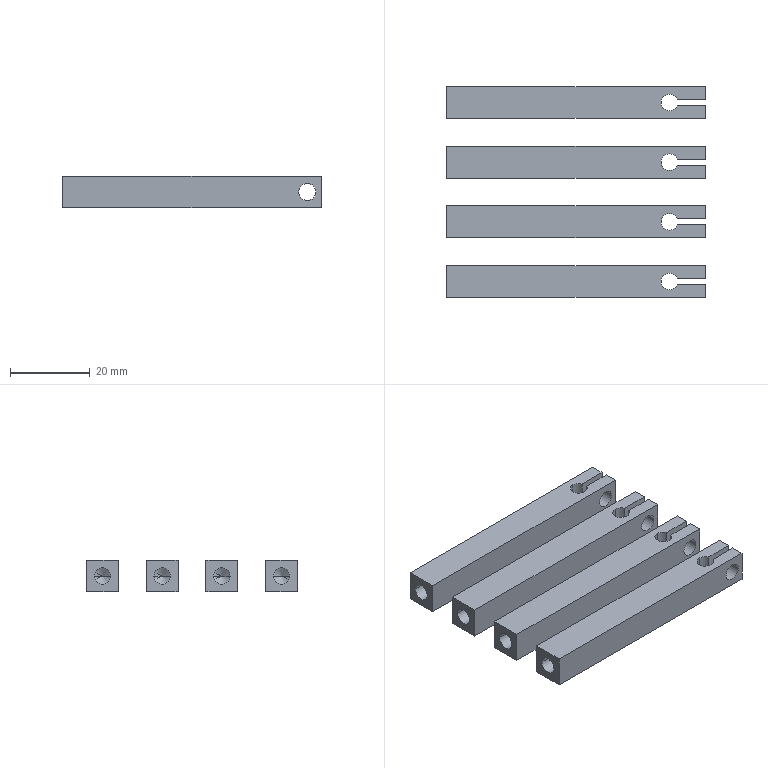CAM job | NX | 3+2 milling, drilling | part box 65 x 53 x 8 mm | stock box 69 x 57 x 9 mm
Tools:
number,name,description,diameter,corner_radius,flute_length,length,flutes
11,D10JING,Milling Tool-5 Parameters,10.0,0.0,50.0,75.0,2
7,D6A45,Milling Tool-5 Parameters,6.0,0.0,50.0,75.0,2
14,4.2ZT,Drilling Tool,4.2,0.0,35.0,50.0,2
6,D6,Milling Tool-5 Parameters,6.0,0.0,50.0,75.0,2
13,D1.5,Milling Tool-5 Parameters,1.5,0.0,50.0,75.0,2
12,4.3ZT,Drilling Tool,4.3,0.0,35.0,50.0,2
Operations:
program,operation,operation_type,tool,method,geometry_group,spindle_rpm,surface_speed,feed_per_tooth,feed_cut,feed_plunge,cut_length_mm,path_length_mm,cut_time_min,machine_time_min
1,FLOOR_WALL,VolumeBased25DMillingOperation,D10JING,METHOD,A,9500.0,298.0,0.0658,1250.0,100.0,1014.997,1068.997,0.812,0.8174
1,DRILLING,Operation,D6A45,METHOD,A,5000.0,94.0,0.025,250.0,0.0,20.8,156.491,0.0832,0.0968
1,DRILLING_COPY_COPY,Operation,4.2ZT,METHOD,A,2000.0,31.0,0.05,200.0,0.0,55.047,224.986,0.2752,0.2922
1,ZLEVEL_PROFILE,ZLevelMilling,D6,METHOD,A,9500.0,179.0,0.1158,2200.0,1000.0,10201.217,10691.591,4.72,4.769
1,PLANAR_PROFILE,PlanarMilling,D1.5,METHOD,A,9500.0,44.0,0.0526,1000.0,100.0,4012.319,25209.319,4.012,6.132
1,PLANAR_MILL_COPY,PlanarMilling,D6A45,METHOD,A,9500.0,179.0,0.0658,1250.0,100.0,680.955,1270.838,0.5448,0.6038
1,ZLEVEL_PROFILE_COPY,ZLevelMilling,D6,METHOD,A,9500.0,298.0,0.0632,1200.0,1000.0,2678.392,3320.693,2.233,2.297
2,DRILLING_COPY,Operation,D6A45,METHOD,B,5000.0,94.0,0.025,250.0,0.0,5.25,70.5,0.021,0.0275
2,DRILLING_COPY_COPY_COPY,Operation,4.3ZT,METHOD,B,2000.0,31.0,0.05,200.0,0.0,12.792,85.584,0.064,0.0712
3,DRILLING_COPY_COPY_1,Operation,D6A45,METHOD,C,5000.0,94.0,0.025,250.0,0.0,5.25,70.5,0.021,0.0275
3,DRILLING_COPY_COPY_COPY_1,Operation,4.2ZT,METHOD,C,2000.0,31.0,0.05,200.0,0.0,16.662,93.324,0.0833,0.091